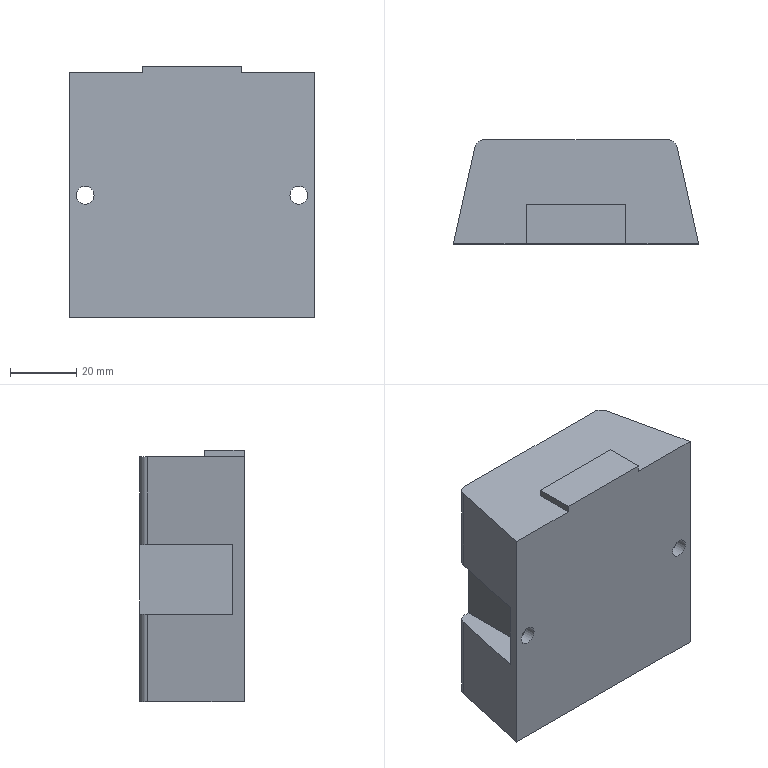Part | NX | features BREP 1 | 1 solid | 24 faces | box 74 x 31.5 x 76 mm | volume 148254 mm3 | plane 18 | cylinder 6 | commonest cylinder face diameters 6 x4 5.4 x2
STEP:
#1=CARTESIAN_POINT('',(34.95,3.5,37.));
#2=VERTEX_POINT('',#1);
#3=CARTESIAN_POINT('',(32.25,3.5,37.));
#4=DIRECTION('',(0.,1.,0.));
#5=DIRECTION('',(1.,0.,0.));
#6=AXIS2_PLACEMENT_3D('',#3,#4,#5);
#7=CIRCLE('',#6,2.7);
#8=EDGE_CURVE('',#2,#2,#7,.T.);
#9=ORIENTED_EDGE('',*,*,#8,.T.);
#10=EDGE_LOOP('',(#9));
#11=FACE_BOUND('',#10,.T.);
#12=CARTESIAN_POINT('',(29.55,0.,37.));
#13=VERTEX_POINT('',#12);
#14=CARTESIAN_POINT('',(32.25,0.,37.));
#15=DIRECTION('',(0.,1.,0.));
#16=DIRECTION('',(-1.,0.,0.));
#17=AXIS2_PLACEMENT_3D('',#14,#15,#16);
#18=CIRCLE('',#17,2.7);
#19=EDGE_CURVE('',#13,#13,#18,.T.);
#20=ORIENTED_EDGE('',*,*,#19,.F.);
#21=EDGE_LOOP('',(#20));
#22=FACE_BOUND('',#21,.T.);
#23=CARTESIAN_POINT('',(32.25,-24.5,37.));
#24=DIRECTION('',(0.,1.,0.));
#25=DIRECTION('',(-1.,0.,0.));
#26=AXIS2_PLACEMENT_3D('',#23,#24,#25);
#27=CYLINDRICAL_SURFACE('',#26,2.7);
#28=ADVANCED_FACE('',(#11,#22),#27,.F.);
#29=CARTESIAN_POINT('',(-34.95,3.5,37.));
#30=VERTEX_POINT('',#29);
#31=CARTESIAN_POINT('',(-32.25,3.5,37.));
#32=DIRECTION('',(0.,1.,0.));
#33=DIRECTION('',(-1.,0.,0.));
#34=AXIS2_PLACEMENT_3D('',#31,#32,#33);
#35=CIRCLE('',#34,2.7);
#36=EDGE_CURVE('',#30,#30,#35,.T.);
#37=ORIENTED_EDGE('',*,*,#36,.T.);
#38=EDGE_LOOP('',(#37));
#39=FACE_BOUND('',#38,.T.);
#40=CARTESIAN_POINT('',(-34.95,0.,37.));
#41=VERTEX_POINT('',#40);
#42=CARTESIAN_POINT('',(-32.25,0.,37.));
#43=DIRECTION('',(0.,1.,0.));
#44=DIRECTION('',(-1.,0.,0.));
#45=AXIS2_PLACEMENT_3D('',#42,#43,#44);
#46=CIRCLE('',#45,2.7);
#47=EDGE_CURVE('',#41,#41,#46,.T.);
#48=ORIENTED_EDGE('',*,*,#47,.F.);
#49=EDGE_LOOP('',(#48));
#50=FACE_BOUND('',#49,.T.);
#51=CARTESIAN_POINT('',(-32.25,-24.5,37.));
#52=DIRECTION('',(0.,1.,0.));
#53=DIRECTION('',(-1.,0.,0.));
#54=AXIS2_PLACEMENT_3D('',#51,#52,#53);
#55=CYLINDRICAL_SURFACE('',#54,2.7);
#56=ADVANCED_FACE('',(#39,#50),#55,.F.);
#57=CARTESIAN_POINT('',(30.522,29.151,26.5));
#58=VERTEX_POINT('',#57);
#59=CARTESIAN_POINT('',(27.593,31.5,26.5));
#60=VERTEX_POINT('',#59);
#61=CARTESIAN_POINT('',(27.593,28.5,26.5));
#62=DIRECTION('',(0.,0.,1.));
#63=DIRECTION('',(-1.,0.,0.));
#64=AXIS2_PLACEMENT_3D('',#61,#62,#63);
#65=CIRCLE('',#64,3.);
#66=EDGE_CURVE('',#58,#60,#65,.T.);
#67=ORIENTED_EDGE('',*,*,#66,.F.);
#68=CARTESIAN_POINT('',(30.522,29.151,0.));
#69=VERTEX_POINT('',#68);
#70=CARTESIAN_POINT('',(30.522,29.151,74.));
#71=DIRECTION('',(0.,0.,1.));
#72=VECTOR('',#71,1000.);
#73=LINE('',#70,#72);
#74=EDGE_CURVE('',#69,#58,#73,.T.);
#75=ORIENTED_EDGE('',*,*,#74,.F.);
#76=CARTESIAN_POINT('',(27.593,31.5,0.));
#77=VERTEX_POINT('',#76);
#78=CARTESIAN_POINT('',(27.593,28.5,0.));
#79=DIRECTION('',(0.,0.,-1.));
#80=DIRECTION('',(-1.,0.,0.));
#81=AXIS2_PLACEMENT_3D('',#78,#79,#80);
#82=CIRCLE('',#81,3.);
#83=EDGE_CURVE('',#77,#69,#82,.T.);
#84=ORIENTED_EDGE('',*,*,#83,.F.);
#85=CARTESIAN_POINT('',(27.593,31.5,74.));
#86=DIRECTION('',(0.,0.,-1.));
#87=VECTOR('',#86,1000.);
#88=LINE('',#85,#87);
#89=EDGE_CURVE('',#60,#77,#88,.T.);
#90=ORIENTED_EDGE('',*,*,#89,.F.);
#91=EDGE_LOOP('',(#67,#75,#84,#90));
#92=FACE_BOUND('',#91,.T.);
#93=CARTESIAN_POINT('',(27.593,28.5,74.));
#94=DIRECTION('',(0.,0.,-1.));
#95=DIRECTION('',(-1.,0.,0.));
#96=AXIS2_PLACEMENT_3D('',#93,#94,#95);
#97=CYLINDRICAL_SURFACE('',#96,3.);
#98=ADVANCED_FACE('',(#92),#97,.T.);
#99=CARTESIAN_POINT('',(-27.593,31.5,26.5));
#100=VERTEX_POINT('',#99);
#101=CARTESIAN_POINT('',(-30.522,29.151,26.5));
#102=VERTEX_POINT('',#101);
#103=CARTESIAN_POINT('',(-27.593,28.5,26.5));
#104=DIRECTION('',(0.,0.,1.));
#105=DIRECTION('',(-1.,0.,0.));
#106=AXIS2_PLACEMENT_3D('',#103,#104,#105);
#107=CIRCLE('',#106,3.);
#108=EDGE_CURVE('',#100,#102,#107,.T.);
#109=ORIENTED_EDGE('',*,*,#108,.F.);
#110=CARTESIAN_POINT('',(-27.593,31.5,0.));
#111=VERTEX_POINT('',#110);
#112=CARTESIAN_POINT('',(-27.593,31.5,74.));
#113=DIRECTION('',(0.,0.,1.));
#114=VECTOR('',#113,1000.);
#115=LINE('',#112,#114);
#116=EDGE_CURVE('',#111,#100,#115,.T.);
#117=ORIENTED_EDGE('',*,*,#116,.F.);
#118=CARTESIAN_POINT('',(-30.522,29.151,0.));
#119=VERTEX_POINT('',#118);
#120=CARTESIAN_POINT('',(-27.593,28.5,0.));
#121=DIRECTION('',(0.,0.,-1.));
#122=DIRECTION('',(-1.,0.,0.));
#123=AXIS2_PLACEMENT_3D('',#120,#121,#122);
#124=CIRCLE('',#123,3.);
#125=EDGE_CURVE('',#119,#111,#124,.T.);
#126=ORIENTED_EDGE('',*,*,#125,.F.);
#127=CARTESIAN_POINT('',(-30.522,29.151,74.));
#128=DIRECTION('',(0.,0.,-1.));
#129=VECTOR('',#128,1000.);
#130=LINE('',#127,#129);
#131=EDGE_CURVE('',#102,#119,#130,.T.);
#132=ORIENTED_EDGE('',*,*,#131,.F.);
#133=EDGE_LOOP('',(#109,#117,#126,#132));
#134=FACE_BOUND('',#133,.T.);
#135=CARTESIAN_POINT('',(-27.593,28.5,74.));
#136=DIRECTION('',(0.,0.,-1.));
#137=DIRECTION('',(-1.,0.,0.));
#138=AXIS2_PLACEMENT_3D('',#135,#136,#137);
#139=CYLINDRICAL_SURFACE('',#138,3.);
#140=ADVANCED_FACE('',(#134),#139,.T.);
#141=CARTESIAN_POINT('',(-15.,12.,74.));
#142=VERTEX_POINT('',#141);
#143=CARTESIAN_POINT('',(-15.,0.,74.));
#144=VERTEX_POINT('',#143);
#145=CARTESIAN_POINT('',(-15.,0.,74.));
#146=DIRECTION('',(0.,-1.,0.));
#147=VECTOR('',#146,1000.);
#148=LINE('',#145,#147);
#149=EDGE_CURVE('',#142,#144,#148,.T.);
#150=ORIENTED_EDGE('',*,*,#149,.F.);
#151=CARTESIAN_POINT('',(15.,12.,74.));
#152=VERTEX_POINT('',#151);
#153=CARTESIAN_POINT('',(-15.,12.,74.));
#154=DIRECTION('',(-1.,0.,0.));
#155=VECTOR('',#154,1000.);
#156=LINE('',#153,#155);
#157=EDGE_CURVE('',#152,#142,#156,.T.);
#158=ORIENTED_EDGE('',*,*,#157,.F.);
#159=CARTESIAN_POINT('',(15.,0.,74.));
#160=VERTEX_POINT('',#159);
#161=CARTESIAN_POINT('',(15.,0.,74.));
#162=DIRECTION('',(0.,1.,0.));
#163=VECTOR('',#162,1000.);
#164=LINE('',#161,#163);
#165=EDGE_CURVE('',#160,#152,#164,.T.);
#166=ORIENTED_EDGE('',*,*,#165,.F.);
#167=CARTESIAN_POINT('',(37.,0.,74.));
#168=VERTEX_POINT('',#167);
#169=CARTESIAN_POINT('',(37.,0.,74.));
#170=DIRECTION('',(1.,0.,0.));
#171=VECTOR('',#170,1000.);
#172=LINE('',#169,#171);
#173=EDGE_CURVE('',#160,#168,#172,.T.);
#174=ORIENTED_EDGE('',*,*,#173,.T.);
#175=CARTESIAN_POINT('',(30.522,29.151,74.));
#176=VERTEX_POINT('',#175);
#177=CARTESIAN_POINT('',(30.,31.5,74.));
#178=DIRECTION('',(-0.2169,0.9762,0.));
#179=VECTOR('',#178,1000.);
#180=LINE('',#177,#179);
#181=EDGE_CURVE('',#168,#176,#180,.T.);
#182=ORIENTED_EDGE('',*,*,#181,.T.);
#183=CARTESIAN_POINT('',(27.593,31.5,74.));
#184=VERTEX_POINT('',#183);
#185=CARTESIAN_POINT('',(27.593,28.5,74.));
#186=DIRECTION('',(0.,0.,1.));
#187=DIRECTION('',(-1.,0.,0.));
#188=AXIS2_PLACEMENT_3D('',#185,#186,#187);
#189=CIRCLE('',#188,3.);
#190=EDGE_CURVE('',#176,#184,#189,.T.);
#191=ORIENTED_EDGE('',*,*,#190,.T.);
#192=CARTESIAN_POINT('',(-27.593,31.5,74.));
#193=VERTEX_POINT('',#192);
#194=CARTESIAN_POINT('',(-30.,31.5,74.));
#195=DIRECTION('',(-1.,0.,0.));
#196=VECTOR('',#195,1000.);
#197=LINE('',#194,#196);
#198=EDGE_CURVE('',#184,#193,#197,.T.);
#199=ORIENTED_EDGE('',*,*,#198,.T.);
#200=CARTESIAN_POINT('',(-30.522,29.151,74.));
#201=VERTEX_POINT('',#200);
#202=CARTESIAN_POINT('',(-27.593,28.5,74.));
#203=DIRECTION('',(0.,0.,1.));
#204=DIRECTION('',(-1.,0.,0.));
#205=AXIS2_PLACEMENT_3D('',#202,#203,#204);
#206=CIRCLE('',#205,3.);
#207=EDGE_CURVE('',#193,#201,#206,.T.);
#208=ORIENTED_EDGE('',*,*,#207,.T.);
#209=CARTESIAN_POINT('',(-37.,0.,74.));
#210=VERTEX_POINT('',#209);
#211=CARTESIAN_POINT('',(-30.,31.5,74.));
#212=DIRECTION('',(-0.2169,-0.9762,0.));
#213=VECTOR('',#212,1000.);
#214=LINE('',#211,#213);
#215=EDGE_CURVE('',#201,#210,#214,.T.);
#216=ORIENTED_EDGE('',*,*,#215,.T.);
#217=CARTESIAN_POINT('',(37.,0.,74.));
#218=DIRECTION('',(1.,0.,0.));
#219=VECTOR('',#218,1000.);
#220=LINE('',#217,#219);
#221=EDGE_CURVE('',#210,#144,#220,.T.);
#222=ORIENTED_EDGE('',*,*,#221,.T.);
#223=EDGE_LOOP('',(#150,#158,#166,#174,#182,#191,#199,#208,#216,#222));
#224=FACE_BOUND('',#223,.T.);
#225=CARTESIAN_POINT('',(0.,0.,74.));
#226=DIRECTION('',(0.,0.,-1.));
#227=DIRECTION('',(-1.,0.,0.));
#228=AXIS2_PLACEMENT_3D('',#225,#226,#227);
#229=PLANE('',#228);
#230=ADVANCED_FACE('',(#224),#229,.F.);
#231=ORIENTED_EDGE('',*,*,#74,.T.);
#232=CARTESIAN_POINT('',(36.222,3.5,26.5));
#233=VERTEX_POINT('',#232);
#234=CARTESIAN_POINT('',(30.,31.5,26.5));
#235=DIRECTION('',(0.2169,-0.9762,0.));
#236=VECTOR('',#235,1000.);
#237=LINE('',#234,#236);
#238=EDGE_CURVE('',#58,#233,#237,.T.);
#239=ORIENTED_EDGE('',*,*,#238,.T.);
#240=CARTESIAN_POINT('',(36.222,3.5,47.5));
#241=VERTEX_POINT('',#240);
#242=CARTESIAN_POINT('',(36.222,3.5,74.));
#243=DIRECTION('',(0.,0.,-1.));
#244=VECTOR('',#243,1000.);
#245=LINE('',#242,#244);
#246=EDGE_CURVE('',#241,#233,#245,.T.);
#247=ORIENTED_EDGE('',*,*,#246,.F.);
#248=CARTESIAN_POINT('',(30.522,29.151,47.5));
#249=VERTEX_POINT('',#248);
#250=CARTESIAN_POINT('',(30.,31.5,47.5));
#251=DIRECTION('',(-0.2169,0.9762,0.));
#252=VECTOR('',#251,1000.);
#253=LINE('',#250,#252);
#254=EDGE_CURVE('',#241,#249,#253,.T.);
#255=ORIENTED_EDGE('',*,*,#254,.T.);
#256=CARTESIAN_POINT('',(30.522,29.151,74.));
#257=DIRECTION('',(0.,0.,1.));
#258=VECTOR('',#257,1000.);
#259=LINE('',#256,#258);
#260=EDGE_CURVE('',#249,#176,#259,.T.);
#261=ORIENTED_EDGE('',*,*,#260,.T.);
#262=ORIENTED_EDGE('',*,*,#181,.F.);
#263=CARTESIAN_POINT('',(37.,0.,0.));
#264=VERTEX_POINT('',#263);
#265=CARTESIAN_POINT('',(37.,0.,74.));
#266=DIRECTION('',(0.,0.,-1.));
#267=VECTOR('',#266,1000.);
#268=LINE('',#265,#267);
#269=EDGE_CURVE('',#168,#264,#268,.T.);
#270=ORIENTED_EDGE('',*,*,#269,.T.);
#271=CARTESIAN_POINT('',(30.,31.5,0.));
#272=DIRECTION('',(-0.2169,0.9762,0.));
#273=VECTOR('',#272,1000.);
#274=LINE('',#271,#273);
#275=EDGE_CURVE('',#264,#69,#274,.T.);
#276=ORIENTED_EDGE('',*,*,#275,.T.);
#277=EDGE_LOOP('',(#231,#239,#247,#255,#261,#262,#270,#276));
#278=FACE_BOUND('',#277,.T.);
#279=CARTESIAN_POINT('',(30.,31.5,74.));
#280=DIRECTION('',(-0.9762,-0.2169,0.));
#281=DIRECTION('',(0.2169,-0.9762,0.));
#282=AXIS2_PLACEMENT_3D('',#279,#280,#281);
#283=PLANE('',#282);
#284=ADVANCED_FACE('',(#278),#283,.F.);
#285=CARTESIAN_POINT('',(26.,31.5,26.5));
#286=VERTEX_POINT('',#285);
#287=CARTESIAN_POINT('',(26.,31.5,47.5));
#288=VERTEX_POINT('',#287);
#289=CARTESIAN_POINT('',(26.,31.5,26.5));
#290=DIRECTION('',(0.,0.,1.));
#291=VECTOR('',#290,1000.);
#292=LINE('',#289,#291);
#293=EDGE_CURVE('',#286,#288,#292,.T.);
#294=ORIENTED_EDGE('',*,*,#293,.F.);
#295=CARTESIAN_POINT('',(37.,31.5,26.5));
#296=DIRECTION('',(-1.,0.,0.));
#297=VECTOR('',#296,1000.);
#298=LINE('',#295,#297);
#299=EDGE_CURVE('',#60,#286,#298,.T.);
#300=ORIENTED_EDGE('',*,*,#299,.F.);
#301=ORIENTED_EDGE('',*,*,#89,.T.);
#302=CARTESIAN_POINT('',(-30.,31.5,0.));
#303=DIRECTION('',(-1.,0.,0.));
#304=VECTOR('',#303,1000.);
#305=LINE('',#302,#304);
#306=EDGE_CURVE('',#77,#111,#305,.T.);
#307=ORIENTED_EDGE('',*,*,#306,.T.);
#308=ORIENTED_EDGE('',*,*,#116,.T.);
#309=CARTESIAN_POINT('',(-26.,31.5,26.5));
#310=VERTEX_POINT('',#309);
#311=CARTESIAN_POINT('',(-37.,31.5,26.5));
#312=DIRECTION('',(-1.,0.,0.));
#313=VECTOR('',#312,1000.);
#314=LINE('',#311,#313);
#315=EDGE_CURVE('',#310,#100,#314,.T.);
#316=ORIENTED_EDGE('',*,*,#315,.F.);
#317=CARTESIAN_POINT('',(-26.,31.5,47.5));
#318=VERTEX_POINT('',#317);
#319=CARTESIAN_POINT('',(-26.,31.5,26.5));
#320=DIRECTION('',(0.,0.,-1.));
#321=VECTOR('',#320,1000.);
#322=LINE('',#319,#321);
#323=EDGE_CURVE('',#318,#310,#322,.T.);
#324=ORIENTED_EDGE('',*,*,#323,.F.);
#325=CARTESIAN_POINT('',(-27.593,31.5,47.5));
#326=VERTEX_POINT('',#325);
#327=CARTESIAN_POINT('',(-37.,31.5,47.5));
#328=DIRECTION('',(1.,0.,0.));
#329=VECTOR('',#328,1000.);
#330=LINE('',#327,#329);
#331=EDGE_CURVE('',#326,#318,#330,.T.);
#332=ORIENTED_EDGE('',*,*,#331,.F.);
#333=CARTESIAN_POINT('',(-27.593,31.5,74.));
#334=DIRECTION('',(0.,0.,1.));
#335=VECTOR('',#334,1000.);
#336=LINE('',#333,#335);
#337=EDGE_CURVE('',#326,#193,#336,.T.);
#338=ORIENTED_EDGE('',*,*,#337,.T.);
#339=ORIENTED_EDGE('',*,*,#198,.F.);
#340=CARTESIAN_POINT('',(27.593,31.5,47.5));
#341=VERTEX_POINT('',#340);
#342=CARTESIAN_POINT('',(27.593,31.5,74.));
#343=DIRECTION('',(0.,0.,-1.));
#344=VECTOR('',#343,1000.);
#345=LINE('',#342,#344);
#346=EDGE_CURVE('',#184,#341,#345,.T.);
#347=ORIENTED_EDGE('',*,*,#346,.T.);
#348=CARTESIAN_POINT('',(37.,31.5,47.5));
#349=DIRECTION('',(1.,0.,0.));
#350=VECTOR('',#349,1000.);
#351=LINE('',#348,#350);
#352=EDGE_CURVE('',#288,#341,#351,.T.);
#353=ORIENTED_EDGE('',*,*,#352,.F.);
#354=EDGE_LOOP('',(#294,#300,#301,#307,#308,#316,#324,#332,#338,#339,#347,#353));
#355=FACE_BOUND('',#354,.T.);
#356=CARTESIAN_POINT('',(-30.,31.5,74.));
#357=DIRECTION('',(0.,-1.,0.));
#358=DIRECTION('',(1.,0.,0.));
#359=AXIS2_PLACEMENT_3D('',#356,#357,#358);
#360=PLANE('',#359);
#361=ADVANCED_FACE('',(#355),#360,.F.);
#362=CARTESIAN_POINT('',(-36.222,3.5,26.5));
#363=VERTEX_POINT('',#362);
#364=CARTESIAN_POINT('',(-36.222,3.5,47.5));
#365=VERTEX_POINT('',#364);
#366=CARTESIAN_POINT('',(-36.222,3.5,74.));
#367=DIRECTION('',(0.,0.,1.));
#368=VECTOR('',#367,1000.);
#369=LINE('',#366,#368);
#370=EDGE_CURVE('',#363,#365,#369,.T.);
#371=ORIENTED_EDGE('',*,*,#370,.F.);
#372=CARTESIAN_POINT('',(-30.,31.5,26.5));
#373=DIRECTION('',(0.2169,0.9762,0.));
#374=VECTOR('',#373,1000.);
#375=LINE('',#372,#374);
#376=EDGE_CURVE('',#363,#102,#375,.T.);
#377=ORIENTED_EDGE('',*,*,#376,.T.);
#378=ORIENTED_EDGE('',*,*,#131,.T.);
#379=CARTESIAN_POINT('',(-37.,0.,0.));
#380=VERTEX_POINT('',#379);
#381=CARTESIAN_POINT('',(-30.,31.5,0.));
#382=DIRECTION('',(-0.2169,-0.9762,0.));
#383=VECTOR('',#382,1000.);
#384=LINE('',#381,#383);
#385=EDGE_CURVE('',#119,#380,#384,.T.);
#386=ORIENTED_EDGE('',*,*,#385,.T.);
#387=CARTESIAN_POINT('',(-37.,0.,74.));
#388=DIRECTION('',(0.,0.,-1.));
#389=VECTOR('',#388,1000.);
#390=LINE('',#387,#389);
#391=EDGE_CURVE('',#210,#380,#390,.T.);
#392=ORIENTED_EDGE('',*,*,#391,.F.);
#393=ORIENTED_EDGE('',*,*,#215,.F.);
#394=CARTESIAN_POINT('',(-30.522,29.151,47.5));
#395=VERTEX_POINT('',#394);
#396=CARTESIAN_POINT('',(-30.522,29.151,74.));
#397=DIRECTION('',(0.,0.,-1.));
#398=VECTOR('',#397,1000.);
#399=LINE('',#396,#398);
#400=EDGE_CURVE('',#201,#395,#399,.T.);
#401=ORIENTED_EDGE('',*,*,#400,.T.);
#402=CARTESIAN_POINT('',(-30.,31.5,47.5));
#403=DIRECTION('',(-0.2169,-0.9762,0.));
#404=VECTOR('',#403,1000.);
#405=LINE('',#402,#404);
#406=EDGE_CURVE('',#395,#365,#405,.T.);
#407=ORIENTED_EDGE('',*,*,#406,.T.);
#408=EDGE_LOOP('',(#371,#377,#378,#386,#392,#393,#401,#407));
#409=FACE_BOUND('',#408,.T.);
#410=CARTESIAN_POINT('',(-30.,31.5,74.));
#411=DIRECTION('',(0.9762,-0.2169,0.));
#412=DIRECTION('',(0.2169,0.9762,0.));
#413=AXIS2_PLACEMENT_3D('',#410,#411,#412);
#414=PLANE('',#413);
#415=ADVANCED_FACE('',(#409),#414,.F.);
#416=ORIENTED_EDGE('',*,*,#19,.T.);
#417=EDGE_LOOP('',(#416));
#418=FACE_BOUND('',#417,.T.);
#419=ORIENTED_EDGE('',*,*,#47,.T.);
#420=EDGE_LOOP('',(#419));
#421=FACE_BOUND('',#420,.T.);
#422=CARTESIAN_POINT('',(37.,0.,0.));
#423=DIRECTION('',(1.,0.,0.));
#424=VECTOR('',#423,1000.);
#425=LINE('',#422,#424);
#426=EDGE_CURVE('',#380,#264,#425,.T.);
#427=ORIENTED_EDGE('',*,*,#426,.T.);
#428=ORIENTED_EDGE('',*,*,#269,.F.);
#429=ORIENTED_EDGE('',*,*,#173,.F.);
#430=CARTESIAN_POINT('',(15.,0.,76.));
#431=VERTEX_POINT('',#430);
#432=CARTESIAN_POINT('',(15.,0.,76.));
#433=DIRECTION('',(0.,0.,-1.));
#434=VECTOR('',#433,1000.);
#435=LINE('',#432,#434);
#436=EDGE_CURVE('',#431,#160,#435,.T.);
#437=ORIENTED_EDGE('',*,*,#436,.F.);
#438=CARTESIAN_POINT('',(-15.,0.,76.));
#439=VERTEX_POINT('',#438);
#440=CARTESIAN_POINT('',(-15.,0.,76.));
#441=DIRECTION('',(1.,0.,0.));
#442=VECTOR('',#441,1000.);
#443=LINE('',#440,#442);
#444=EDGE_CURVE('',#439,#431,#443,.T.);
#445=ORIENTED_EDGE('',*,*,#444,.F.);
#446=CARTESIAN_POINT('',(-15.,0.,76.));
#447=DIRECTION('',(0.,0.,-1.));
#448=VECTOR('',#447,1000.);
#449=LINE('',#446,#448);
#450=EDGE_CURVE('',#439,#144,#449,.T.);
#451=ORIENTED_EDGE('',*,*,#450,.T.);
#452=ORIENTED_EDGE('',*,*,#221,.F.);
#453=ORIENTED_EDGE('',*,*,#391,.T.);
#454=EDGE_LOOP('',(#427,#428,#429,#437,#445,#451,#452,#453));
#455=FACE_BOUND('',#454,.T.);
#456=CARTESIAN_POINT('',(37.,0.,74.));
#457=DIRECTION('',(0.,1.,0.));
#458=DIRECTION('',(-1.,0.,0.));
#459=AXIS2_PLACEMENT_3D('',#456,#457,#458);
#460=PLANE('',#459);
#461=ADVANCED_FACE('',(#418,#421,#455),#460,.F.);
#462=ORIENTED_EDGE('',*,*,#385,.F.);
#463=ORIENTED_EDGE('',*,*,#125,.T.);
#464=ORIENTED_EDGE('',*,*,#306,.F.);
#465=ORIENTED_EDGE('',*,*,#83,.T.);
#466=ORIENTED_EDGE('',*,*,#275,.F.);
#467=ORIENTED_EDGE('',*,*,#426,.F.);
#468=EDGE_LOOP('',(#462,#463,#464,#465,#466,#467));
#469=FACE_BOUND('',#468,.T.);
#470=CARTESIAN_POINT('',(0.,0.,0.));
#471=DIRECTION('',(0.,0.,-1.));
#472=DIRECTION('',(-1.,0.,0.));
#473=AXIS2_PLACEMENT_3D('',#470,#471,#472);
#474=PLANE('',#473);
#475=ADVANCED_FACE('',(#469),#474,.T.);
#476=CARTESIAN_POINT('',(-27.593,28.5,47.5));
#477=DIRECTION('',(0.,0.,-1.));
#478=DIRECTION('',(1.,0.,0.));
#479=AXIS2_PLACEMENT_3D('',#476,#477,#478);
#480=CIRCLE('',#479,3.);
#481=EDGE_CURVE('',#395,#326,#480,.T.);
#482=ORIENTED_EDGE('',*,*,#481,.F.);
#483=ORIENTED_EDGE('',*,*,#400,.F.);
#484=ORIENTED_EDGE('',*,*,#207,.F.);
#485=ORIENTED_EDGE('',*,*,#337,.F.);
#486=EDGE_LOOP('',(#482,#483,#484,#485));
#487=FACE_BOUND('',#486,.T.);
#488=CARTESIAN_POINT('',(-27.593,28.5,74.));
#489=DIRECTION('',(0.,0.,-1.));
#490=DIRECTION('',(-1.,0.,0.));
#491=AXIS2_PLACEMENT_3D('',#488,#489,#490);
#492=CYLINDRICAL_SURFACE('',#491,3.);
#493=ADVANCED_FACE('',(#487),#492,.T.);
#494=CARTESIAN_POINT('',(27.593,28.5,47.5));
#495=DIRECTION('',(0.,0.,-1.));
#496=DIRECTION('',(1.,0.,0.));
#497=AXIS2_PLACEMENT_3D('',#494,#495,#496);
#498=CIRCLE('',#497,3.);
#499=EDGE_CURVE('',#341,#249,#498,.T.);
#500=ORIENTED_EDGE('',*,*,#499,.F.);
#501=ORIENTED_EDGE('',*,*,#346,.F.);
#502=ORIENTED_EDGE('',*,*,#190,.F.);
#503=ORIENTED_EDGE('',*,*,#260,.F.);
#504=EDGE_LOOP('',(#500,#501,#502,#503));
#505=FACE_BOUND('',#504,.T.);
#506=CARTESIAN_POINT('',(27.593,28.5,74.));
#507=DIRECTION('',(0.,0.,-1.));
#508=DIRECTION('',(-1.,0.,0.));
#509=AXIS2_PLACEMENT_3D('',#506,#507,#508);
#510=CYLINDRICAL_SURFACE('',#509,3.);
#511=ADVANCED_FACE('',(#505),#510,.T.);
#512=ORIENTED_EDGE('',*,*,#149,.T.);
#513=ORIENTED_EDGE('',*,*,#450,.F.);
#514=CARTESIAN_POINT('',(-15.,12.,76.));
#515=VERTEX_POINT('',#514);
#516=CARTESIAN_POINT('',(-15.,0.,76.));
#517=DIRECTION('',(0.,-1.,0.));
#518=VECTOR('',#517,1000.);
#519=LINE('',#516,#518);
#520=EDGE_CURVE('',#515,#439,#519,.T.);
#521=ORIENTED_EDGE('',*,*,#520,.F.);
#522=CARTESIAN_POINT('',(-15.,12.,76.));
#523=DIRECTION('',(0.,0.,-1.));
#524=VECTOR('',#523,1000.);
#525=LINE('',#522,#524);
#526=EDGE_CURVE('',#515,#142,#525,.T.);
#527=ORIENTED_EDGE('',*,*,#526,.T.);
#528=EDGE_LOOP('',(#512,#513,#521,#527));
#529=FACE_BOUND('',#528,.T.);
#530=CARTESIAN_POINT('',(-15.,0.,76.));
#531=DIRECTION('',(1.,0.,0.));
#532=DIRECTION('',(0.,1.,0.));
#533=AXIS2_PLACEMENT_3D('',#530,#531,#532);
#534=PLANE('',#533);
#535=ADVANCED_FACE('',(#529),#534,.F.);
#536=ORIENTED_EDGE('',*,*,#165,.T.);
#537=CARTESIAN_POINT('',(15.,12.,76.));
#538=VERTEX_POINT('',#537);
#539=CARTESIAN_POINT('',(15.,12.,76.));
#540=DIRECTION('',(0.,0.,-1.));
#541=VECTOR('',#540,1000.);
#542=LINE('',#539,#541);
#543=EDGE_CURVE('',#538,#152,#542,.T.);
#544=ORIENTED_EDGE('',*,*,#543,.F.);
#545=CARTESIAN_POINT('',(15.,0.,76.));
#546=DIRECTION('',(0.,1.,0.));
#547=VECTOR('',#546,1000.);
#548=LINE('',#545,#547);
#549=EDGE_CURVE('',#431,#538,#548,.T.);
#550=ORIENTED_EDGE('',*,*,#549,.F.);
#551=ORIENTED_EDGE('',*,*,#436,.T.);
#552=EDGE_LOOP('',(#536,#544,#550,#551));
#553=FACE_BOUND('',#552,.T.);
#554=CARTESIAN_POINT('',(15.,0.,76.));
#555=DIRECTION('',(-1.,0.,0.));
#556=DIRECTION('',(0.,0.,1.));
#557=AXIS2_PLACEMENT_3D('',#554,#555,#556);
#558=PLANE('',#557);
#559=ADVANCED_FACE('',(#553),#558,.F.);
#560=ORIENTED_EDGE('',*,*,#157,.T.);
#561=ORIENTED_EDGE('',*,*,#526,.F.);
#562=CARTESIAN_POINT('',(-15.,12.,76.));
#563=DIRECTION('',(-1.,0.,0.));
#564=VECTOR('',#563,1000.);
#565=LINE('',#562,#564);
#566=EDGE_CURVE('',#538,#515,#565,.T.);
#567=ORIENTED_EDGE('',*,*,#566,.F.);
#568=ORIENTED_EDGE('',*,*,#543,.T.);
#569=EDGE_LOOP('',(#560,#561,#567,#568));
#570=FACE_BOUND('',#569,.T.);
#571=CARTESIAN_POINT('',(-15.,12.,76.));
#572=DIRECTION('',(0.,-1.,0.));
#573=DIRECTION('',(1.,0.,0.));
#574=AXIS2_PLACEMENT_3D('',#571,#572,#573);
#575=PLANE('',#574);
#576=ADVANCED_FACE('',(#570),#575,.F.);
#577=ORIENTED_EDGE('',*,*,#520,.T.);
#578=ORIENTED_EDGE('',*,*,#444,.T.);
#579=ORIENTED_EDGE('',*,*,#549,.T.);
#580=ORIENTED_EDGE('',*,*,#566,.T.);
#581=EDGE_LOOP('',(#577,#578,#579,#580));
#582=FACE_BOUND('',#581,.T.);
#583=CARTESIAN_POINT('',(0.,0.,76.));
#584=DIRECTION('',(0.,0.,-1.));
#585=DIRECTION('',(-1.,0.,0.));
#586=AXIS2_PLACEMENT_3D('',#583,#584,#585);
#587=PLANE('',#586);
#588=ADVANCED_FACE('',(#582),#587,.F.);
#589=ORIENTED_EDGE('',*,*,#36,.F.);
#590=EDGE_LOOP('',(#589));
#591=FACE_BOUND('',#590,.T.);
#592=ORIENTED_EDGE('',*,*,#370,.T.);
#593=CARTESIAN_POINT('',(-26.,3.5,47.5));
#594=VERTEX_POINT('',#593);
#595=CARTESIAN_POINT('',(-37.,3.5,47.5));
#596=DIRECTION('',(1.,0.,0.));
#597=VECTOR('',#596,1000.);
#598=LINE('',#595,#597);
#599=EDGE_CURVE('',#365,#594,#598,.T.);
#600=ORIENTED_EDGE('',*,*,#599,.T.);
#601=CARTESIAN_POINT('',(-26.,3.5,26.5));
#602=VERTEX_POINT('',#601);
#603=CARTESIAN_POINT('',(-26.,3.5,26.5));
#604=DIRECTION('',(0.,0.,-1.));
#605=VECTOR('',#604,1000.);
#606=LINE('',#603,#605);
#607=EDGE_CURVE('',#594,#602,#606,.T.);
#608=ORIENTED_EDGE('',*,*,#607,.T.);
#609=CARTESIAN_POINT('',(-37.,3.5,26.5));
#610=DIRECTION('',(-1.,0.,0.));
#611=VECTOR('',#610,1000.);
#612=LINE('',#609,#611);
#613=EDGE_CURVE('',#602,#363,#612,.T.);
#614=ORIENTED_EDGE('',*,*,#613,.T.);
#615=EDGE_LOOP('',(#592,#600,#608,#614));
#616=FACE_BOUND('',#615,.T.);
#617=CARTESIAN_POINT('',(0.,3.5,0.));
#618=DIRECTION('',(0.,1.,0.));
#619=DIRECTION('',(-1.,0.,0.));
#620=AXIS2_PLACEMENT_3D('',#617,#618,#619);
#621=PLANE('',#620);
#622=ADVANCED_FACE('',(#591,#616),#621,.T.);
#623=ORIENTED_EDGE('',*,*,#613,.F.);
#624=CARTESIAN_POINT('',(-26.,3.5,26.5));
#625=DIRECTION('',(0.,1.,0.));
#626=VECTOR('',#625,1000.);
#627=LINE('',#624,#626);
#628=EDGE_CURVE('',#602,#310,#627,.T.);
#629=ORIENTED_EDGE('',*,*,#628,.T.);
#630=ORIENTED_EDGE('',*,*,#315,.T.);
#631=ORIENTED_EDGE('',*,*,#108,.T.);
#632=ORIENTED_EDGE('',*,*,#376,.F.);
#633=EDGE_LOOP('',(#623,#629,#630,#631,#632));
#634=FACE_BOUND('',#633,.T.);
#635=CARTESIAN_POINT('',(-37.,3.5,26.5));
#636=DIRECTION('',(0.,0.,-1.));
#637=DIRECTION('',(-1.,0.,0.));
#638=AXIS2_PLACEMENT_3D('',#635,#636,#637);
#639=PLANE('',#638);
#640=ADVANCED_FACE('',(#634),#639,.F.);
#641=ORIENTED_EDGE('',*,*,#481,.T.);
#642=ORIENTED_EDGE('',*,*,#331,.T.);
#643=CARTESIAN_POINT('',(-26.,3.5,47.5));
#644=DIRECTION('',(0.,1.,0.));
#645=VECTOR('',#644,1000.);
#646=LINE('',#643,#645);
#647=EDGE_CURVE('',#594,#318,#646,.T.);
#648=ORIENTED_EDGE('',*,*,#647,.F.);
#649=ORIENTED_EDGE('',*,*,#599,.F.);
#650=ORIENTED_EDGE('',*,*,#406,.F.);
#651=EDGE_LOOP('',(#641,#642,#648,#649,#650));
#652=FACE_BOUND('',#651,.T.);
#653=CARTESIAN_POINT('',(-37.,3.5,47.5));
#654=DIRECTION('',(0.,0.,1.));
#655=DIRECTION('',(1.,0.,0.));
#656=AXIS2_PLACEMENT_3D('',#653,#654,#655);
#657=PLANE('',#656);
#658=ADVANCED_FACE('',(#652),#657,.F.);
#659=ORIENTED_EDGE('',*,*,#323,.T.);
#660=ORIENTED_EDGE('',*,*,#628,.F.);
#661=ORIENTED_EDGE('',*,*,#607,.F.);
#662=ORIENTED_EDGE('',*,*,#647,.T.);
#663=EDGE_LOOP('',(#659,#660,#661,#662));
#664=FACE_BOUND('',#663,.T.);
#665=CARTESIAN_POINT('',(-26.,3.5,26.5));
#666=DIRECTION('',(1.,0.,0.));
#667=DIRECTION('',(0.,0.,-1.));
#668=AXIS2_PLACEMENT_3D('',#665,#666,#667);
#669=PLANE('',#668);
#670=ADVANCED_FACE('',(#664),#669,.F.);
#671=ORIENTED_EDGE('',*,*,#8,.F.);
#672=EDGE_LOOP('',(#671));
#673=FACE_BOUND('',#672,.T.);
#674=ORIENTED_EDGE('',*,*,#246,.T.);
#675=CARTESIAN_POINT('',(26.,3.5,26.5));
#676=VERTEX_POINT('',#675);
#677=CARTESIAN_POINT('',(37.,3.5,26.5));
#678=DIRECTION('',(-1.,0.,0.));
#679=VECTOR('',#678,1000.);
#680=LINE('',#677,#679);
#681=EDGE_CURVE('',#233,#676,#680,.T.);
#682=ORIENTED_EDGE('',*,*,#681,.T.);
#683=CARTESIAN_POINT('',(26.,3.5,47.5));
#684=VERTEX_POINT('',#683);
#685=CARTESIAN_POINT('',(26.,3.5,26.5));
#686=DIRECTION('',(0.,0.,1.));
#687=VECTOR('',#686,1000.);
#688=LINE('',#685,#687);
#689=EDGE_CURVE('',#676,#684,#688,.T.);
#690=ORIENTED_EDGE('',*,*,#689,.T.);
#691=CARTESIAN_POINT('',(37.,3.5,47.5));
#692=DIRECTION('',(1.,0.,0.));
#693=VECTOR('',#692,1000.);
#694=LINE('',#691,#693);
#695=EDGE_CURVE('',#684,#241,#694,.T.);
#696=ORIENTED_EDGE('',*,*,#695,.T.);
#697=EDGE_LOOP('',(#674,#682,#690,#696));
#698=FACE_BOUND('',#697,.T.);
#699=CARTESIAN_POINT('',(0.,3.5,0.));
#700=DIRECTION('',(0.,1.,0.));
#701=DIRECTION('',(-1.,0.,0.));
#702=AXIS2_PLACEMENT_3D('',#699,#700,#701);
#703=PLANE('',#702);
#704=ADVANCED_FACE('',(#673,#698),#703,.T.);
#705=ORIENTED_EDGE('',*,*,#66,.T.);
#706=ORIENTED_EDGE('',*,*,#299,.T.);
#707=CARTESIAN_POINT('',(26.,3.5,26.5));
#708=DIRECTION('',(0.,1.,0.));
#709=VECTOR('',#708,1000.);
#710=LINE('',#707,#709);
#711=EDGE_CURVE('',#676,#286,#710,.T.);
#712=ORIENTED_EDGE('',*,*,#711,.F.);
#713=ORIENTED_EDGE('',*,*,#681,.F.);
#714=ORIENTED_EDGE('',*,*,#238,.F.);
#715=EDGE_LOOP('',(#705,#706,#712,#713,#714));
#716=FACE_BOUND('',#715,.T.);
#717=CARTESIAN_POINT('',(37.,3.5,26.5));
#718=DIRECTION('',(0.,0.,-1.));
#719=DIRECTION('',(-1.,0.,0.));
#720=AXIS2_PLACEMENT_3D('',#717,#718,#719);
#721=PLANE('',#720);
#722=ADVANCED_FACE('',(#716),#721,.F.);
#723=ORIENTED_EDGE('',*,*,#695,.F.);
#724=CARTESIAN_POINT('',(26.,3.5,47.5));
#725=DIRECTION('',(0.,1.,0.));
#726=VECTOR('',#725,1000.);
#727=LINE('',#724,#726);
#728=EDGE_CURVE('',#684,#288,#727,.T.);
#729=ORIENTED_EDGE('',*,*,#728,.T.);
#730=ORIENTED_EDGE('',*,*,#352,.T.);
#731=ORIENTED_EDGE('',*,*,#499,.T.);
#732=ORIENTED_EDGE('',*,*,#254,.F.);
#733=EDGE_LOOP('',(#723,#729,#730,#731,#732));
#734=FACE_BOUND('',#733,.T.);
#735=CARTESIAN_POINT('',(37.,3.5,47.5));
#736=DIRECTION('',(0.,0.,1.));
#737=DIRECTION('',(1.,0.,0.));
#738=AXIS2_PLACEMENT_3D('',#735,#736,#737);
#739=PLANE('',#738);
#740=ADVANCED_FACE('',(#734),#739,.F.);
#741=ORIENTED_EDGE('',*,*,#293,.T.);
#742=ORIENTED_EDGE('',*,*,#728,.F.);
#743=ORIENTED_EDGE('',*,*,#689,.F.);
#744=ORIENTED_EDGE('',*,*,#711,.T.);
#745=EDGE_LOOP('',(#741,#742,#743,#744));
#746=FACE_BOUND('',#745,.T.);
#747=CARTESIAN_POINT('',(26.,3.5,26.5));
#748=DIRECTION('',(-1.,0.,0.));
#749=DIRECTION('',(0.,0.,1.));
#750=AXIS2_PLACEMENT_3D('',#747,#748,#749);
#751=PLANE('',#750);
#752=ADVANCED_FACE('',(#746),#751,.F.);
#753=CLOSED_SHELL('',(#28,#56,#98,#140,#230,#284,#361,#415,#461,#475,#493,#511,#535,#559,#576,#588,#622,#640,#658,#670,#704,#722,#740,#752));
#754=MANIFOLD_SOLID_BREP('',#753);
#755=(LENGTH_UNIT()NAMED_UNIT(*)SI_UNIT(.MILLI.,.METRE.));
#756=UNCERTAINTY_MEASURE_WITH_UNIT(LENGTH_MEASURE(0.00001),#755,'','');
#757=(NAMED_UNIT(*)PLANE_ANGLE_UNIT()SI_UNIT($,.RADIAN.));
#758=(NAMED_UNIT(*)SI_UNIT($,.STERADIAN.)SOLID_ANGLE_UNIT());
#759=(GEOMETRIC_REPRESENTATION_CONTEXT(3)GLOBAL_UNCERTAINTY_ASSIGNED_CONTEXT((#756))GLOBAL_UNIT_ASSIGNED_CONTEXT((#755,#757,#758))REPRESENTATION_CONTEXT('',''));
#760=ADVANCED_BREP_SHAPE_REPRESENTATION('',(#754),#759);